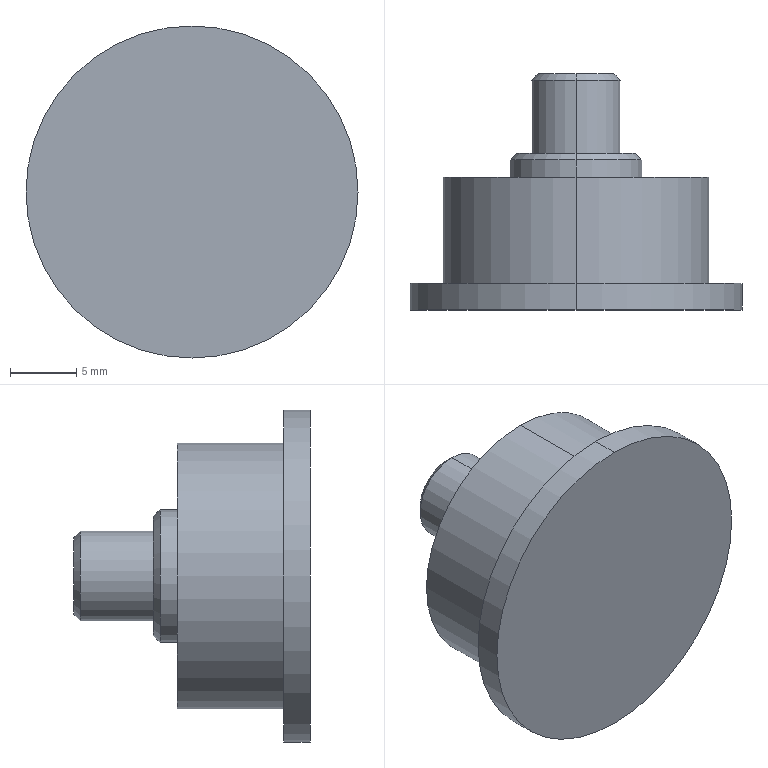Part | SolidWorks | features Chamfer 1, Revolution 1 | 1 solid | 17 faces | box 25 x 17.8 x 25 mm | volume 3845 mm3 | cylinder 8 | plane 5 | cone 4 | commonest cylinder face diameters 6.746 x2 10 x2 20 x2 25 x2
STEP:
#1=CARTESIAN_POINT('',(24.234,-54.531,2.873));
#2=VERTEX_POINT('',#1);
#3=CARTESIAN_POINT('',(24.234,-54.531,-2.873));
#4=VERTEX_POINT('',#3);
#5=CARTESIAN_POINT('',(24.234,-54.531,0.));
#6=DIRECTION('',(0.,1.,0.));
#7=DIRECTION('',(0.,0.,1.));
#8=AXIS2_PLACEMENT_3D('',#5,#6,#7);
#9=CIRCLE('',#8,2.873);
#10=EDGE_CURVE('',#2,#4,#9,.T.);
#11=ORIENTED_EDGE('',*,*,#10,.F.);
#12=CARTESIAN_POINT('',(24.234,-55.031,3.373));
#13=VERTEX_POINT('',#12);
#14=CARTESIAN_POINT('',(24.234,-54.531,2.873));
#15=DIRECTION('',(0.,-0.7071,0.7071));
#16=VECTOR('',#15,1000.);
#17=LINE('',#14,#16);
#18=EDGE_CURVE('',#2,#13,#17,.T.);
#19=ORIENTED_EDGE('',*,*,#18,.T.);
#20=CARTESIAN_POINT('',(24.234,-55.031,-3.373));
#21=VERTEX_POINT('',#20);
#22=CARTESIAN_POINT('',(24.234,-55.031,0.));
#23=DIRECTION('',(0.,-1.,0.));
#24=DIRECTION('',(0.,0.,1.));
#25=AXIS2_PLACEMENT_3D('',#22,#23,#24);
#26=CIRCLE('',#25,3.373);
#27=EDGE_CURVE('',#21,#13,#26,.T.);
#28=ORIENTED_EDGE('',*,*,#27,.F.);
#29=CARTESIAN_POINT('',(24.234,-54.531,-2.873));
#30=DIRECTION('',(0.,-0.7071,-0.7071));
#31=VECTOR('',#30,1000.);
#32=LINE('',#29,#31);
#33=EDGE_CURVE('',#4,#21,#32,.T.);
#34=ORIENTED_EDGE('',*,*,#33,.F.);
#35=EDGE_LOOP('',(#11,#19,#28,#34));
#36=FACE_OUTER_BOUND('',#35,.T.);
#37=CARTESIAN_POINT('',(24.234,-54.531,0.));
#38=DIRECTION('',(0.,-1.,0.));
#39=DIRECTION('',(0.,0.,-1.));
#40=AXIS2_PLACEMENT_3D('',#37,#38,#39);
#41=CONICAL_SURFACE('',#40,2.873,0.7854);
#42=ADVANCED_FACE('',(#36),#41,.T.);
#43=CARTESIAN_POINT('',(24.234,-60.531,4.5));
#44=VERTEX_POINT('',#43);
#45=CARTESIAN_POINT('',(24.234,-60.531,-4.5));
#46=VERTEX_POINT('',#45);
#47=CARTESIAN_POINT('',(24.234,-60.531,0.));
#48=DIRECTION('',(0.,1.,0.));
#49=DIRECTION('',(0.,0.,1.));
#50=AXIS2_PLACEMENT_3D('',#47,#48,#49);
#51=CIRCLE('',#50,4.5);
#52=EDGE_CURVE('',#44,#46,#51,.T.);
#53=ORIENTED_EDGE('',*,*,#52,.F.);
#54=CARTESIAN_POINT('',(24.234,-61.031,5.));
#55=VERTEX_POINT('',#54);
#56=CARTESIAN_POINT('',(24.234,-60.531,4.5));
#57=DIRECTION('',(0.,-0.7071,0.7071));
#58=VECTOR('',#57,1000.);
#59=LINE('',#56,#58);
#60=EDGE_CURVE('',#44,#55,#59,.T.);
#61=ORIENTED_EDGE('',*,*,#60,.T.);
#62=CARTESIAN_POINT('',(24.234,-61.031,-5.));
#63=VERTEX_POINT('',#62);
#64=CARTESIAN_POINT('',(24.234,-61.031,0.));
#65=DIRECTION('',(0.,-1.,0.));
#66=DIRECTION('',(0.,0.,1.));
#67=AXIS2_PLACEMENT_3D('',#64,#65,#66);
#68=CIRCLE('',#67,5.);
#69=EDGE_CURVE('',#63,#55,#68,.T.);
#70=ORIENTED_EDGE('',*,*,#69,.F.);
#71=CARTESIAN_POINT('',(24.234,-60.531,-4.5));
#72=DIRECTION('',(0.,-0.7071,-0.7071));
#73=VECTOR('',#72,1000.);
#74=LINE('',#71,#73);
#75=EDGE_CURVE('',#46,#63,#74,.T.);
#76=ORIENTED_EDGE('',*,*,#75,.F.);
#77=EDGE_LOOP('',(#53,#61,#70,#76));
#78=FACE_OUTER_BOUND('',#77,.T.);
#79=CARTESIAN_POINT('',(24.234,-60.531,0.));
#80=DIRECTION('',(0.,-1.,0.));
#81=DIRECTION('',(0.,0.,-1.));
#82=AXIS2_PLACEMENT_3D('',#79,#80,#81);
#83=CONICAL_SURFACE('',#82,4.5,0.7854);
#84=ADVANCED_FACE('',(#78),#83,.T.);
#85=CARTESIAN_POINT('',(24.234,-60.531,3.373));
#86=VERTEX_POINT('',#85);
#87=CARTESIAN_POINT('',(24.234,-60.531,-3.373));
#88=VERTEX_POINT('',#87);
#89=CARTESIAN_POINT('',(24.234,-60.531,0.));
#90=DIRECTION('',(0.,1.,0.));
#91=DIRECTION('',(0.,0.,1.));
#92=AXIS2_PLACEMENT_3D('',#89,#90,#91);
#93=CIRCLE('',#92,3.373);
#94=EDGE_CURVE('',#86,#88,#93,.T.);
#95=ORIENTED_EDGE('',*,*,#94,.T.);
#96=CARTESIAN_POINT('',(24.234,-52.031,-3.373));
#97=DIRECTION('',(0.,1.,0.));
#98=VECTOR('',#97,1000.);
#99=LINE('',#96,#98);
#100=EDGE_CURVE('',#88,#21,#99,.T.);
#101=ORIENTED_EDGE('',*,*,#100,.T.);
#102=ORIENTED_EDGE('',*,*,#27,.T.);
#103=CARTESIAN_POINT('',(24.234,-52.031,3.373));
#104=DIRECTION('',(0.,1.,0.));
#105=VECTOR('',#104,1000.);
#106=LINE('',#103,#105);
#107=EDGE_CURVE('',#86,#13,#106,.T.);
#108=ORIENTED_EDGE('',*,*,#107,.F.);
#109=EDGE_LOOP('',(#95,#101,#102,#108));
#110=FACE_OUTER_BOUND('',#109,.T.);
#111=CARTESIAN_POINT('',(24.234,-52.031,0.));
#112=DIRECTION('',(0.,1.,0.));
#113=DIRECTION('',(0.,0.,1.));
#114=AXIS2_PLACEMENT_3D('',#111,#112,#113);
#115=CYLINDRICAL_SURFACE('',#114,3.373);
#116=ADVANCED_FACE('',(#110),#115,.T.);
#117=CARTESIAN_POINT('',(24.234,-62.331,5.));
#118=VERTEX_POINT('',#117);
#119=CARTESIAN_POINT('',(24.234,-62.331,-5.));
#120=VERTEX_POINT('',#119);
#121=CARTESIAN_POINT('',(24.234,-62.331,0.));
#122=DIRECTION('',(0.,1.,0.));
#123=DIRECTION('',(0.,0.,1.));
#124=AXIS2_PLACEMENT_3D('',#121,#122,#123);
#125=CIRCLE('',#124,5.);
#126=EDGE_CURVE('',#118,#120,#125,.T.);
#127=ORIENTED_EDGE('',*,*,#126,.T.);
#128=CARTESIAN_POINT('',(24.234,-52.031,-5.));
#129=DIRECTION('',(0.,1.,0.));
#130=VECTOR('',#129,1000.);
#131=LINE('',#128,#130);
#132=EDGE_CURVE('',#120,#63,#131,.T.);
#133=ORIENTED_EDGE('',*,*,#132,.T.);
#134=ORIENTED_EDGE('',*,*,#69,.T.);
#135=CARTESIAN_POINT('',(24.234,-52.031,5.));
#136=DIRECTION('',(0.,1.,0.));
#137=VECTOR('',#136,1000.);
#138=LINE('',#135,#137);
#139=EDGE_CURVE('',#118,#55,#138,.T.);
#140=ORIENTED_EDGE('',*,*,#139,.F.);
#141=EDGE_LOOP('',(#127,#133,#134,#140));
#142=FACE_OUTER_BOUND('',#141,.T.);
#143=CARTESIAN_POINT('',(24.234,-52.031,0.));
#144=DIRECTION('',(0.,1.,0.));
#145=DIRECTION('',(0.,0.,1.));
#146=AXIS2_PLACEMENT_3D('',#143,#144,#145);
#147=CYLINDRICAL_SURFACE('',#146,5.);
#148=ADVANCED_FACE('',(#142),#147,.T.);
#149=CARTESIAN_POINT('',(24.234,-70.331,10.));
#150=VERTEX_POINT('',#149);
#151=CARTESIAN_POINT('',(24.234,-70.331,-10.));
#152=VERTEX_POINT('',#151);
#153=CARTESIAN_POINT('',(24.234,-70.331,0.));
#154=DIRECTION('',(0.,1.,0.));
#155=DIRECTION('',(0.,0.,1.));
#156=AXIS2_PLACEMENT_3D('',#153,#154,#155);
#157=CIRCLE('',#156,10.);
#158=EDGE_CURVE('',#150,#152,#157,.T.);
#159=ORIENTED_EDGE('',*,*,#158,.T.);
#160=CARTESIAN_POINT('',(24.234,-62.331,-10.));
#161=VERTEX_POINT('',#160);
#162=CARTESIAN_POINT('',(24.234,-52.031,-10.));
#163=DIRECTION('',(0.,1.,0.));
#164=VECTOR('',#163,1000.);
#165=LINE('',#162,#164);
#166=EDGE_CURVE('',#152,#161,#165,.T.);
#167=ORIENTED_EDGE('',*,*,#166,.T.);
#168=CARTESIAN_POINT('',(24.234,-62.331,10.));
#169=VERTEX_POINT('',#168);
#170=CARTESIAN_POINT('',(24.234,-62.331,0.));
#171=DIRECTION('',(0.,1.,0.));
#172=DIRECTION('',(0.,0.,1.));
#173=AXIS2_PLACEMENT_3D('',#170,#171,#172);
#174=CIRCLE('',#173,10.);
#175=EDGE_CURVE('',#169,#161,#174,.T.);
#176=ORIENTED_EDGE('',*,*,#175,.F.);
#177=CARTESIAN_POINT('',(24.234,-52.031,10.));
#178=DIRECTION('',(0.,1.,0.));
#179=VECTOR('',#178,1000.);
#180=LINE('',#177,#179);
#181=EDGE_CURVE('',#150,#169,#180,.T.);
#182=ORIENTED_EDGE('',*,*,#181,.F.);
#183=EDGE_LOOP('',(#159,#167,#176,#182));
#184=FACE_OUTER_BOUND('',#183,.T.);
#185=CARTESIAN_POINT('',(24.234,-52.031,0.));
#186=DIRECTION('',(0.,1.,0.));
#187=DIRECTION('',(0.,0.,1.));
#188=AXIS2_PLACEMENT_3D('',#185,#186,#187);
#189=CYLINDRICAL_SURFACE('',#188,10.);
#190=ADVANCED_FACE('',(#184),#189,.T.);
#191=CARTESIAN_POINT('',(24.234,-72.331,12.5));
#192=VERTEX_POINT('',#191);
#193=CARTESIAN_POINT('',(24.234,-72.331,-12.5));
#194=VERTEX_POINT('',#193);
#195=CARTESIAN_POINT('',(24.234,-72.331,0.));
#196=DIRECTION('',(0.,1.,0.));
#197=DIRECTION('',(0.,0.,1.));
#198=AXIS2_PLACEMENT_3D('',#195,#196,#197);
#199=CIRCLE('',#198,12.5);
#200=EDGE_CURVE('',#192,#194,#199,.T.);
#201=ORIENTED_EDGE('',*,*,#200,.T.);
#202=CARTESIAN_POINT('',(24.234,-70.331,-12.5));
#203=VERTEX_POINT('',#202);
#204=CARTESIAN_POINT('',(24.234,-52.031,-12.5));
#205=DIRECTION('',(0.,1.,0.));
#206=VECTOR('',#205,1000.);
#207=LINE('',#204,#206);
#208=EDGE_CURVE('',#194,#203,#207,.T.);
#209=ORIENTED_EDGE('',*,*,#208,.T.);
#210=CARTESIAN_POINT('',(24.234,-70.331,12.5));
#211=VERTEX_POINT('',#210);
#212=CARTESIAN_POINT('',(24.234,-70.331,0.));
#213=DIRECTION('',(0.,1.,0.));
#214=DIRECTION('',(0.,0.,1.));
#215=AXIS2_PLACEMENT_3D('',#212,#213,#214);
#216=CIRCLE('',#215,12.5);
#217=EDGE_CURVE('',#211,#203,#216,.T.);
#218=ORIENTED_EDGE('',*,*,#217,.F.);
#219=CARTESIAN_POINT('',(24.234,-52.031,12.5));
#220=DIRECTION('',(0.,1.,0.));
#221=VECTOR('',#220,1000.);
#222=LINE('',#219,#221);
#223=EDGE_CURVE('',#192,#211,#222,.T.);
#224=ORIENTED_EDGE('',*,*,#223,.F.);
#225=EDGE_LOOP('',(#201,#209,#218,#224));
#226=FACE_OUTER_BOUND('',#225,.T.);
#227=CARTESIAN_POINT('',(24.234,-52.031,0.));
#228=DIRECTION('',(0.,1.,0.));
#229=DIRECTION('',(0.,0.,1.));
#230=AXIS2_PLACEMENT_3D('',#227,#228,#229);
#231=CYLINDRICAL_SURFACE('',#230,12.5);
#232=ADVANCED_FACE('',(#226),#231,.T.);
#233=ORIENTED_EDGE('',*,*,#200,.F.);
#234=CARTESIAN_POINT('',(24.234,-72.331,0.));
#235=DIRECTION('',(0.,1.,0.));
#236=DIRECTION('',(0.,0.,1.));
#237=AXIS2_PLACEMENT_3D('',#234,#235,#236);
#238=CIRCLE('',#237,12.5);
#239=EDGE_CURVE('',#194,#192,#238,.T.);
#240=ORIENTED_EDGE('',*,*,#239,.F.);
#241=EDGE_LOOP('',(#233,#240));
#242=FACE_OUTER_BOUND('',#241,.T.);
#243=CARTESIAN_POINT('',(11.734,-72.331,0.));
#244=DIRECTION('',(0.,-1.,0.));
#245=DIRECTION('',(0.,0.,-1.));
#246=AXIS2_PLACEMENT_3D('',#243,#244,#245);
#247=PLANE('',#246);
#248=ADVANCED_FACE('',(#242),#247,.T.);
#249=ORIENTED_EDGE('',*,*,#208,.F.);
#250=ORIENTED_EDGE('',*,*,#239,.T.);
#251=ORIENTED_EDGE('',*,*,#223,.T.);
#252=CARTESIAN_POINT('',(24.234,-70.331,0.));
#253=DIRECTION('',(0.,1.,0.));
#254=DIRECTION('',(0.,0.,1.));
#255=AXIS2_PLACEMENT_3D('',#252,#253,#254);
#256=CIRCLE('',#255,12.5);
#257=EDGE_CURVE('',#203,#211,#256,.T.);
#258=ORIENTED_EDGE('',*,*,#257,.F.);
#259=EDGE_LOOP('',(#249,#250,#251,#258));
#260=FACE_OUTER_BOUND('',#259,.T.);
#261=CARTESIAN_POINT('',(24.234,-52.031,0.));
#262=DIRECTION('',(0.,1.,0.));
#263=DIRECTION('',(0.,0.,1.));
#264=AXIS2_PLACEMENT_3D('',#261,#262,#263);
#265=CYLINDRICAL_SURFACE('',#264,12.5);
#266=ADVANCED_FACE('',(#260),#265,.T.);
#267=ORIENTED_EDGE('',*,*,#217,.T.);
#268=ORIENTED_EDGE('',*,*,#257,.T.);
#269=EDGE_LOOP('',(#267,#268));
#270=FACE_OUTER_BOUND('',#269,.T.);
#271=ORIENTED_EDGE('',*,*,#158,.F.);
#272=CARTESIAN_POINT('',(24.234,-70.331,0.));
#273=DIRECTION('',(0.,1.,0.));
#274=DIRECTION('',(0.,0.,1.));
#275=AXIS2_PLACEMENT_3D('',#272,#273,#274);
#276=CIRCLE('',#275,10.);
#277=EDGE_CURVE('',#152,#150,#276,.T.);
#278=ORIENTED_EDGE('',*,*,#277,.F.);
#279=EDGE_LOOP('',(#271,#278));
#280=FACE_BOUND('',#279,.T.);
#281=CARTESIAN_POINT('',(14.234,-70.331,0.));
#282=DIRECTION('',(0.,1.,0.));
#283=DIRECTION('',(0.,0.,1.));
#284=AXIS2_PLACEMENT_3D('',#281,#282,#283);
#285=PLANE('',#284);
#286=ADVANCED_FACE('',(#270,#280),#285,.T.);
#287=ORIENTED_EDGE('',*,*,#166,.F.);
#288=ORIENTED_EDGE('',*,*,#277,.T.);
#289=ORIENTED_EDGE('',*,*,#181,.T.);
#290=CARTESIAN_POINT('',(24.234,-62.331,0.));
#291=DIRECTION('',(0.,1.,0.));
#292=DIRECTION('',(0.,0.,1.));
#293=AXIS2_PLACEMENT_3D('',#290,#291,#292);
#294=CIRCLE('',#293,10.);
#295=EDGE_CURVE('',#161,#169,#294,.T.);
#296=ORIENTED_EDGE('',*,*,#295,.F.);
#297=EDGE_LOOP('',(#287,#288,#289,#296));
#298=FACE_OUTER_BOUND('',#297,.T.);
#299=CARTESIAN_POINT('',(24.234,-52.031,0.));
#300=DIRECTION('',(0.,1.,0.));
#301=DIRECTION('',(0.,0.,1.));
#302=AXIS2_PLACEMENT_3D('',#299,#300,#301);
#303=CYLINDRICAL_SURFACE('',#302,10.);
#304=ADVANCED_FACE('',(#298),#303,.T.);
#305=ORIENTED_EDGE('',*,*,#175,.T.);
#306=ORIENTED_EDGE('',*,*,#295,.T.);
#307=EDGE_LOOP('',(#305,#306));
#308=FACE_OUTER_BOUND('',#307,.T.);
#309=ORIENTED_EDGE('',*,*,#126,.F.);
#310=CARTESIAN_POINT('',(24.234,-62.331,0.));
#311=DIRECTION('',(0.,1.,0.));
#312=DIRECTION('',(0.,0.,1.));
#313=AXIS2_PLACEMENT_3D('',#310,#311,#312);
#314=CIRCLE('',#313,5.);
#315=EDGE_CURVE('',#120,#118,#314,.T.);
#316=ORIENTED_EDGE('',*,*,#315,.F.);
#317=EDGE_LOOP('',(#309,#316));
#318=FACE_BOUND('',#317,.T.);
#319=CARTESIAN_POINT('',(19.234,-62.331,0.));
#320=DIRECTION('',(0.,1.,0.));
#321=DIRECTION('',(0.,0.,1.));
#322=AXIS2_PLACEMENT_3D('',#319,#320,#321);
#323=PLANE('',#322);
#324=ADVANCED_FACE('',(#308,#318),#323,.T.);
#325=ORIENTED_EDGE('',*,*,#132,.F.);
#326=ORIENTED_EDGE('',*,*,#315,.T.);
#327=ORIENTED_EDGE('',*,*,#139,.T.);
#328=CARTESIAN_POINT('',(24.234,-61.031,0.));
#329=DIRECTION('',(0.,-1.,0.));
#330=DIRECTION('',(0.,0.,1.));
#331=AXIS2_PLACEMENT_3D('',#328,#329,#330);
#332=CIRCLE('',#331,5.);
#333=EDGE_CURVE('',#55,#63,#332,.T.);
#334=ORIENTED_EDGE('',*,*,#333,.T.);
#335=EDGE_LOOP('',(#325,#326,#327,#334));
#336=FACE_OUTER_BOUND('',#335,.T.);
#337=CARTESIAN_POINT('',(24.234,-52.031,0.));
#338=DIRECTION('',(0.,1.,0.));
#339=DIRECTION('',(0.,0.,1.));
#340=AXIS2_PLACEMENT_3D('',#337,#338,#339);
#341=CYLINDRICAL_SURFACE('',#340,5.);
#342=ADVANCED_FACE('',(#336),#341,.T.);
#343=CARTESIAN_POINT('',(24.234,-60.531,0.));
#344=DIRECTION('',(0.,1.,0.));
#345=DIRECTION('',(0.,0.,1.));
#346=AXIS2_PLACEMENT_3D('',#343,#344,#345);
#347=CIRCLE('',#346,4.5);
#348=EDGE_CURVE('',#46,#44,#347,.T.);
#349=ORIENTED_EDGE('',*,*,#348,.T.);
#350=ORIENTED_EDGE('',*,*,#52,.T.);
#351=EDGE_LOOP('',(#349,#350));
#352=FACE_OUTER_BOUND('',#351,.T.);
#353=ORIENTED_EDGE('',*,*,#94,.F.);
#354=CARTESIAN_POINT('',(24.234,-60.531,0.));
#355=DIRECTION('',(0.,1.,0.));
#356=DIRECTION('',(0.,0.,1.));
#357=AXIS2_PLACEMENT_3D('',#354,#355,#356);
#358=CIRCLE('',#357,3.373);
#359=EDGE_CURVE('',#88,#86,#358,.T.);
#360=ORIENTED_EDGE('',*,*,#359,.F.);
#361=EDGE_LOOP('',(#353,#360));
#362=FACE_BOUND('',#361,.T.);
#363=CARTESIAN_POINT('',(20.861,-60.531,0.));
#364=DIRECTION('',(0.,1.,0.));
#365=DIRECTION('',(0.,0.,1.));
#366=AXIS2_PLACEMENT_3D('',#363,#364,#365);
#367=PLANE('',#366);
#368=ADVANCED_FACE('',(#352,#362),#367,.T.);
#369=ORIENTED_EDGE('',*,*,#100,.F.);
#370=ORIENTED_EDGE('',*,*,#359,.T.);
#371=ORIENTED_EDGE('',*,*,#107,.T.);
#372=CARTESIAN_POINT('',(24.234,-55.031,0.));
#373=DIRECTION('',(0.,-1.,0.));
#374=DIRECTION('',(0.,0.,1.));
#375=AXIS2_PLACEMENT_3D('',#372,#373,#374);
#376=CIRCLE('',#375,3.373);
#377=EDGE_CURVE('',#13,#21,#376,.T.);
#378=ORIENTED_EDGE('',*,*,#377,.T.);
#379=EDGE_LOOP('',(#369,#370,#371,#378));
#380=FACE_OUTER_BOUND('',#379,.T.);
#381=CARTESIAN_POINT('',(24.234,-52.031,0.));
#382=DIRECTION('',(0.,1.,0.));
#383=DIRECTION('',(0.,0.,1.));
#384=AXIS2_PLACEMENT_3D('',#381,#382,#383);
#385=CYLINDRICAL_SURFACE('',#384,3.373);
#386=ADVANCED_FACE('',(#380),#385,.T.);
#387=CARTESIAN_POINT('',(24.234,-54.531,0.));
#388=DIRECTION('',(0.,1.,0.));
#389=DIRECTION('',(0.,0.,1.));
#390=AXIS2_PLACEMENT_3D('',#387,#388,#389);
#391=CIRCLE('',#390,2.873);
#392=EDGE_CURVE('',#4,#2,#391,.T.);
#393=ORIENTED_EDGE('',*,*,#392,.T.);
#394=ORIENTED_EDGE('',*,*,#10,.T.);
#395=EDGE_LOOP('',(#393,#394));
#396=FACE_OUTER_BOUND('',#395,.T.);
#397=CARTESIAN_POINT('',(20.861,-54.531,0.));
#398=DIRECTION('',(0.,1.,0.));
#399=DIRECTION('',(0.,0.,1.));
#400=AXIS2_PLACEMENT_3D('',#397,#398,#399);
#401=PLANE('',#400);
#402=ADVANCED_FACE('',(#396),#401,.T.);
#403=ORIENTED_EDGE('',*,*,#60,.F.);
#404=ORIENTED_EDGE('',*,*,#348,.F.);
#405=ORIENTED_EDGE('',*,*,#75,.T.);
#406=ORIENTED_EDGE('',*,*,#333,.F.);
#407=EDGE_LOOP('',(#403,#404,#405,#406));
#408=FACE_OUTER_BOUND('',#407,.T.);
#409=CARTESIAN_POINT('',(24.234,-60.531,0.));
#410=DIRECTION('',(0.,-1.,0.));
#411=DIRECTION('',(0.,0.,-1.));
#412=AXIS2_PLACEMENT_3D('',#409,#410,#411);
#413=CONICAL_SURFACE('',#412,4.5,0.7854);
#414=ADVANCED_FACE('',(#408),#413,.T.);
#415=ORIENTED_EDGE('',*,*,#18,.F.);
#416=ORIENTED_EDGE('',*,*,#392,.F.);
#417=ORIENTED_EDGE('',*,*,#33,.T.);
#418=ORIENTED_EDGE('',*,*,#377,.F.);
#419=EDGE_LOOP('',(#415,#416,#417,#418));
#420=FACE_OUTER_BOUND('',#419,.T.);
#421=CARTESIAN_POINT('',(24.234,-54.531,0.));
#422=DIRECTION('',(0.,-1.,0.));
#423=DIRECTION('',(0.,0.,-1.));
#424=AXIS2_PLACEMENT_3D('',#421,#422,#423);
#425=CONICAL_SURFACE('',#424,2.873,0.7854);
#426=ADVANCED_FACE('',(#420),#425,.T.);
#427=CLOSED_SHELL('',(#42,#84,#116,#148,#190,#232,#248,#266,#286,#304,#324,#342,#368,#386,#402,#414,#426));
#428=MANIFOLD_SOLID_BREP('',#427);
#429=CARTESIAN_POINT('',(0.,0.,0.));
#430=DIRECTION('',(0.,0.,1.));
#431=DIRECTION('',(1.,0.,0.));
#432=AXIS2_PLACEMENT_3D('',#429,#430,#431);
#433=(LENGTH_UNIT()NAMED_UNIT(*)SI_UNIT(.MILLI.,.METRE.));
#434=UNCERTAINTY_MEASURE_WITH_UNIT(LENGTH_MEASURE(0.00001),#433,'','');
#435=(NAMED_UNIT(*)PLANE_ANGLE_UNIT()SI_UNIT($,.RADIAN.));
#436=(NAMED_UNIT(*)SI_UNIT($,.STERADIAN.)SOLID_ANGLE_UNIT());
#437=(GEOMETRIC_REPRESENTATION_CONTEXT(3)GLOBAL_UNCERTAINTY_ASSIGNED_CONTEXT((#434))GLOBAL_UNIT_ASSIGNED_CONTEXT((#433,#435,#436))REPRESENTATION_CONTEXT('',''));
#438=ADVANCED_BREP_SHAPE_REPRESENTATION('',(#428,#432),#437);